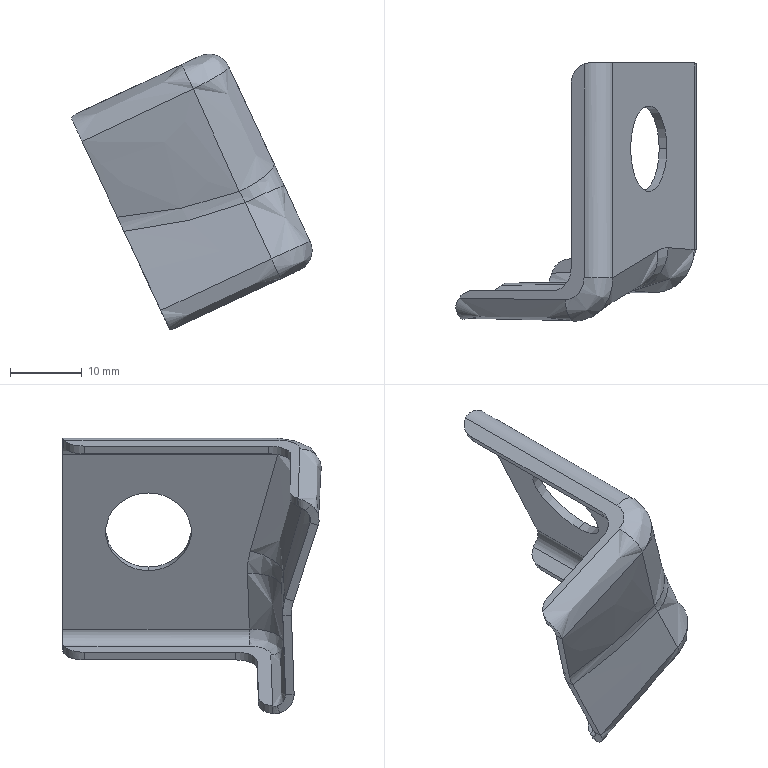Part | STEP file | FNA5401311 | 1 solid | 54 faces | box 33.614 x 36.273 x 38.59 mm | volume 2270 mm3 | spline 35 | plane 11 | cylinder 8 | commonest cylinder face diameters 6 x4 3.6 x2 12 x2